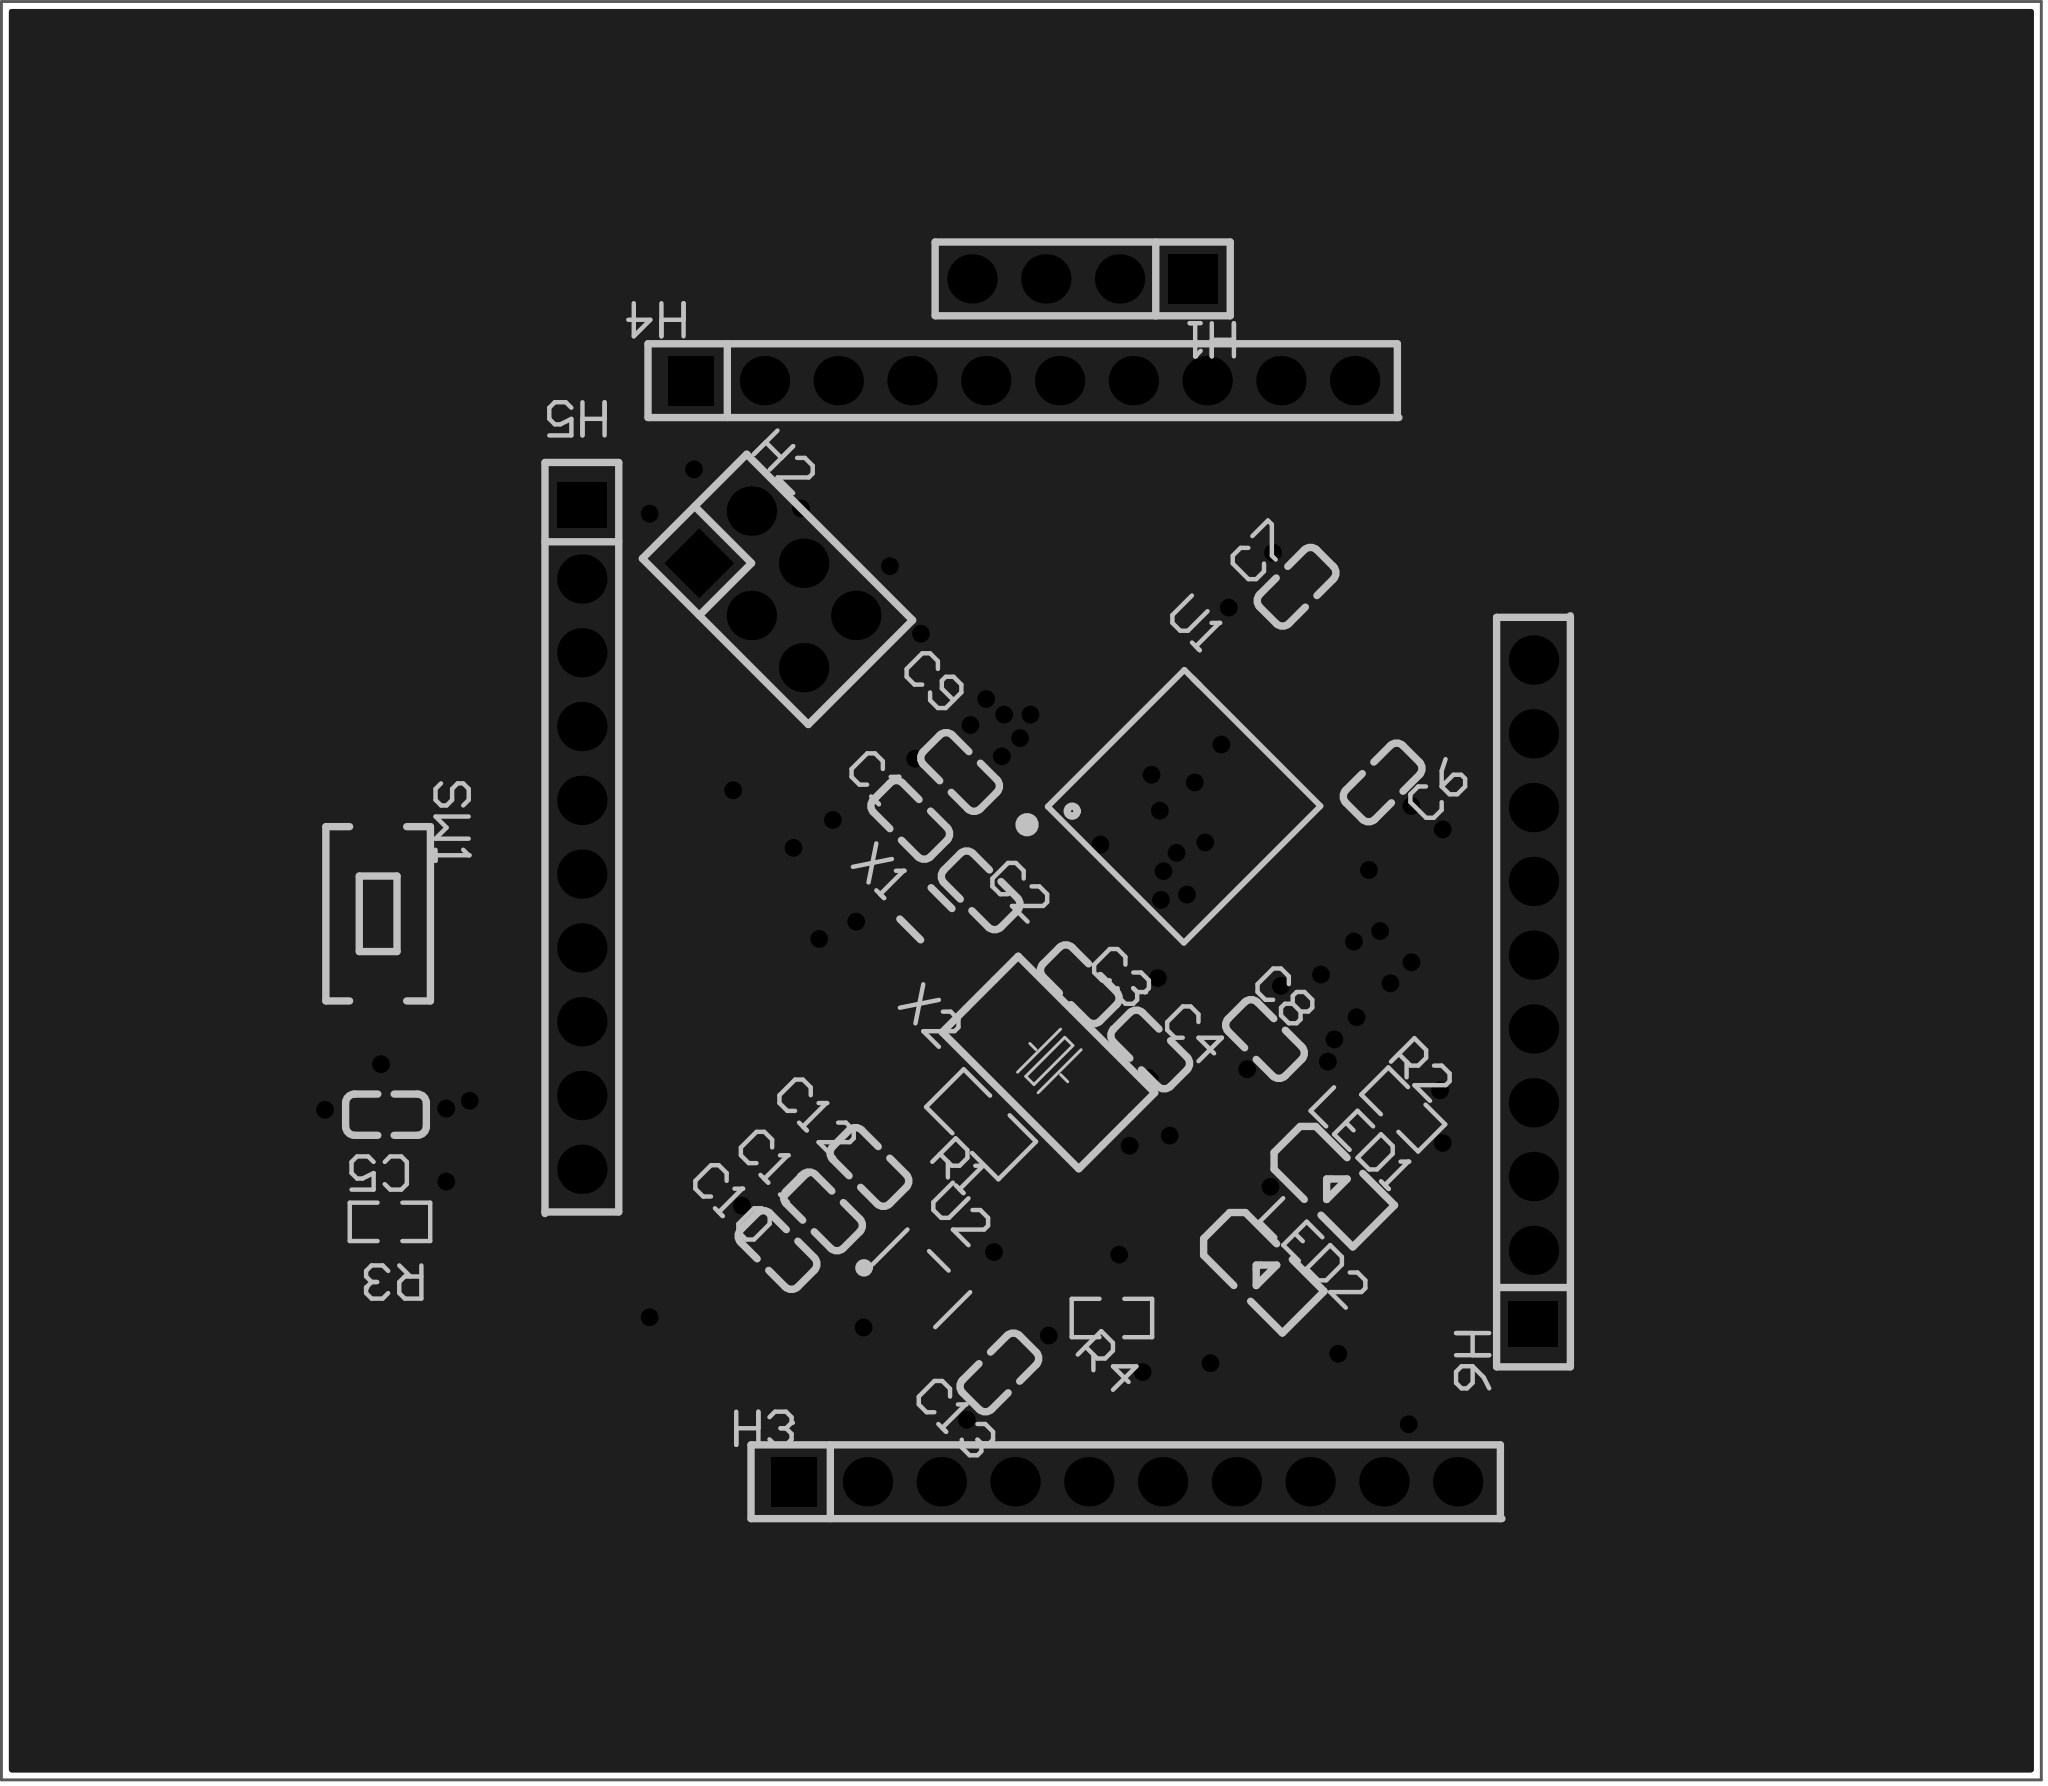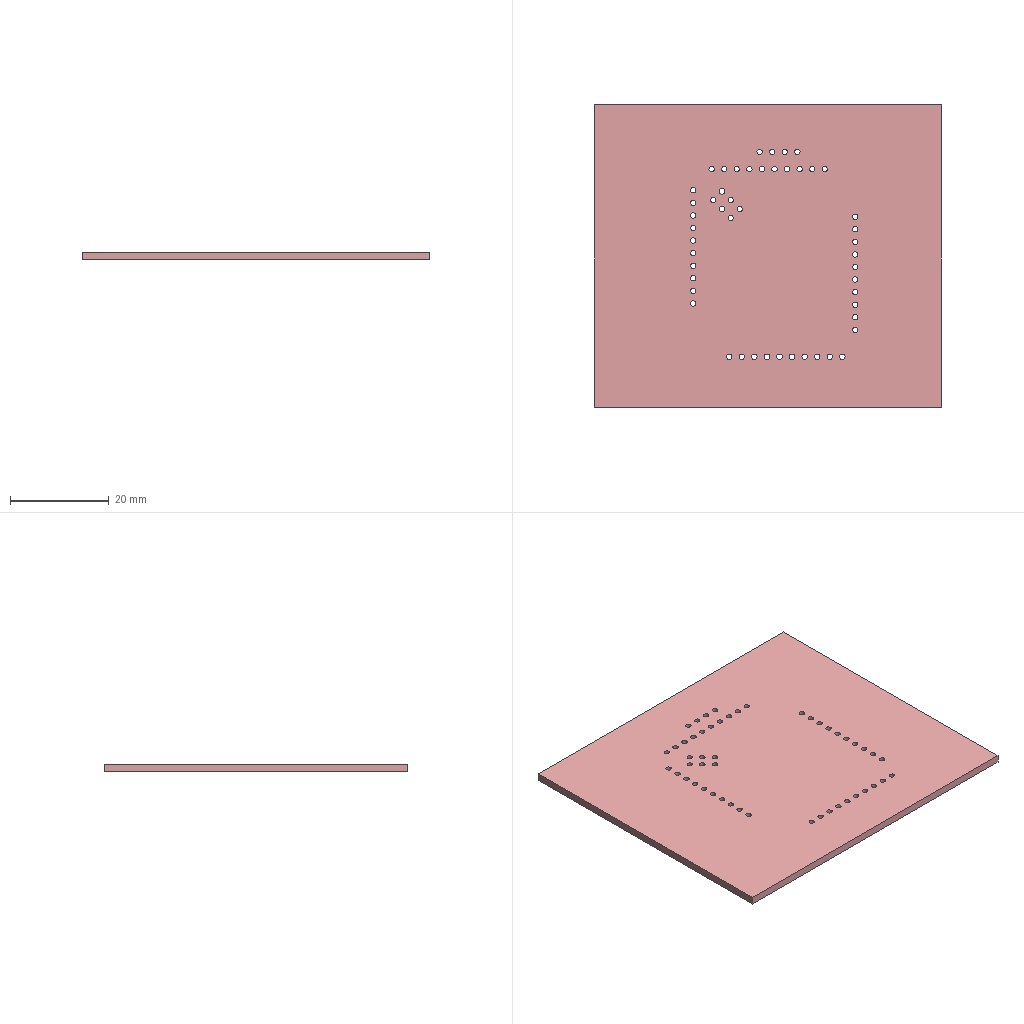Circuit board layout | Altium Designer | box 70.2 x 61.2 x 1.6 mm
Layer stack:
# Altium Designer layer stack of  (unit mm; dielectric type: 0 none, 1 core, 2 prepreg, 3 surface material)
index,name,kind,layer,copper_thickness_mm,dielectric_type,dielectric_thickness_mm,dielectric_material,dielectric_constant
0,Top Paste Mask Layer,other,,,,,,
1,Top Silkscreen Layer,other,,,,,,
2,Top Solder Mask Layer,dielectric,,,3,0.01,,3.3
3,Top Layer,copper,Top Layer,0.035,,,,
4,Dielectric1,dielectric,,,3,1.51,FR4,4.5
5,Bottom Layer,copper,Bottom Layer,0.035,,,,
6,Bottom Solder Mask Layer,dielectric,,,3,0.01,,3.3
7,Bottom Silkscreen Layer,other,,,,,,
8,Bottom Paste Mask Layer,other,,,,,,
# drill layer pairs: low layer,high layer
drill_pair,Top Layer,Bottom Layer
Part placement:
Designator,Comment,Layer,Footprint,Center-X(mm),Center-Y(mm),Rotation
R1,1MΩ,TopLayer,R0805,173.909,165.999,315
R2,510Ω,TopLayer,R0603,188.444,166.51,315
U1,STM32F103C8T6,TopLayer,LQFP-48_L7.0-W7.0-P0.50-LS9.0-BL,180.9,176.927,315
X1,32.768kHz,TopLayer,FC-135R_L3.2-W1.5,172.01,173.245,135
X2,8MHz,TopLayer,CRYSTAL-SMD_L5.0-W3.2,176.23,168.126,135
C1,22pF,TopLayer,C0603,171.471,176.478,315
C2,22pF,TopLayer,C0603,173.895,174.053,135
C3,22pF,TopLayer,C0603,177.308,170.82,315
C4,22pF,TopLayer,C0603,179.733,168.575,135
C5,100nF,TopLayer,C0603,153.421,166.33,0
C6,100nF,TopLayer,C0603,187.735,177.767,225
C7,100nF,TopLayer,C0603,184.771,184.502,225
C8,100nF,TopLayer,C0603,183.684,168.934,315
C9,100nF,TopLayer,C0603,173.187,178.126,315
C12,1uF,TopLayer,C0603,170.066,164.53,315
C13,22nF,TopLayer,C0603,174.538,157.458,45
C11,100nF,TopLayer,C0603,168.468,163.001,315
C10,10uF,TopLayer,C0603,166.901,161.672,315
H1,PZ254V-11-04P,TopLayer,HDR-TH_4P-P2.54-V-M,177.407,195.099,180
H2,PZ254V-12-6P,TopLayer,HDR-TH_6P-P2.54-V-M-R2-C3-S2.54,166.901,184.412,315
H3,PH2.54-1X10P-H25,TopLayer,HDR-TH_10P-P2.54-V-M,178.889,153.695,0
H4,PH2.54-1X10P-H25,TopLayer,HDR-TH_10P-P2.54-V-M,175.342,191.596,0
H5,PH2.54-1X10P-H25,TopLayer,HDR-TH_10P-P2.54-V-M,160.165,175.881,270
H6,PH2.54-1X10P-H25,TopLayer,HDR-TH_10P-P2.54-V-M,192.929,170.55,90
LED1,HL-PSC-2012H233W(6000-7000K),TopLayer,LED0805-R-RD,186.019,163.905,315
LED2,HL-PSC-2012H233W(6000-7000K),TopLayer,LED0805-R-RD,183.594,160.942,315
R3,10kΩ,TopLayer,R0603,153.558,162.641,180
R4,510Ω,TopLayer,R0603,178.415,159.332,180
SW1,TS-1101-C-W,TopLayer,SW-SMD_L6.0-W3.3-LS8.0_TS-1101-C-W,153.151,173.245,270
U2,RT9193-33GB,TopLayer,SOT-23-5_L3.0-W1.7-P0.95-LS2.8-BL,171.853,160.698,315
Pad and via stacks:
# Altium Designer via and pad stacks of  (unit mm). Each distinct definition once, with the count of objects using it.
# via: kind,start_layer,end_layer,hole_mm,diameter_mm,mode(0 simple;1 top-mid-bottom;2 full stack),diameter_per_layer,count,example_net
# pad: kind,layer,hole_mm,hole_type(0 round;1 square;2 slot),plating,top_size,top_shape(1 round;2 rect;3 octagon;9 rounded rect),mid_size,bottom_size,mode,footprint,size_per_layer,count,example
pad,Top Layer,0,0,plated,1.133x1.377,2,1.133x1.377,1.133x1.377,0,R0805,,2,R1.2
pad,Top Layer,0,0,plated,0.8065x0.864,2,0.8065x0.864,0.8065x0.864,0,R0603,,6,R2.2
pad,Top Layer,0,0,plated,0.27x1.5,1,0.27x1.5,0.27x1.5,0,LQFP-48_L7.0-W7.0-P0.50-LS9.0-BL,,24,U1.1
pad,Top Layer,0,0,plated,1.5x0.27,1,1.5x0.27,1.5x0.27,0,LQFP-48_L7.0-W7.0-P0.50-LS9.0-BL,,24,U1.13
pad,Top Layer,0,0,plated,1.8x1,2,1.8x1,1.8x1,0,FC-135R_L3.2-W1.5,,2,X1.1
pad,Top Layer,0,0,plated,1.9x2.4,2,1.9x2.4,1.9x2.4,0,CRYSTAL-SMD_L5.0-W3.2,,2,X2.2
pad,Top Layer,0,0,plated,0.8x0.9,2,0.8x0.9,0.8x0.9,0,C0603,,26,C1.2
pad,Top Layer,0,0,plated,1x1.399,2,1x1.399,1x1.399,0,LED0805-R-RD,,4,LED1.2
pad,Top Layer,0,0,plated,1.2x1,2,1.2x1,1.2x1,0,SW-SMD_L6.0-W3.3-LS8.0_TS-1101-C-W,,2,SW1.1
pad,Top Layer,0,0,plated,0.49x1.157,2,0.49x1.157,0.49x1.157,0,SOT-23-5_L3.0-W1.7-P0.95-LS2.8-BL,,3,U2.1
pad,Top Layer,0,0,plated,0.49x1.175,2,0.49x1.175,0.49x1.175,0,SOT-23-5_L3.0-W1.7-P0.95-LS2.8-BL,,2,U2.4
pad,Multi-Layer,1.1,0,plated,1.7x1.7,2,1.7x1.7,1.7x1.7,0,HDR-TH_4P-P2.54-V-M,,1,H1.1
pad,Multi-Layer,1.1,0,plated,1.7x1.7,1,1.7x1.7,1.7x1.7,0,HDR-TH_4P-P2.54-V-M,,3,H1.2
pad,Multi-Layer,1.1,0,plated,1.7x1.7,2,1.7x1.7,1.7x1.7,0,HDR-TH_6P-P2.54-V-M-R2-C3-S2.54,,1,H2.1
pad,Multi-Layer,1.1,0,plated,1.7x1.7,1,1.7x1.7,1.7x1.7,0,HDR-TH_6P-P2.54-V-M-R2-C3-S2.54,,5,H2.2
pad,Multi-Layer,1.1,0,plated,1.7x1.7,1,1.7x1.7,1.7x1.7,0,HDR-TH_10P-P2.54-V-M,,36,H3.10
pad,Multi-Layer,1.1,0,plated,1.575x1.7,2,1.575x1.7,1.575x1.7,0,HDR-TH_10P-P2.54-V-M,,4,H3.1
via,Top Layer,Bottom Layer,0.3048,0.61,0,,65,BOOT0
Copper pours:
name,layer,net,type(0 solid;1 hatched;2 none)
Bottom Layer-GND,Bottom Layer,GND,0
Top Layer-GND,Top Layer,GND,0